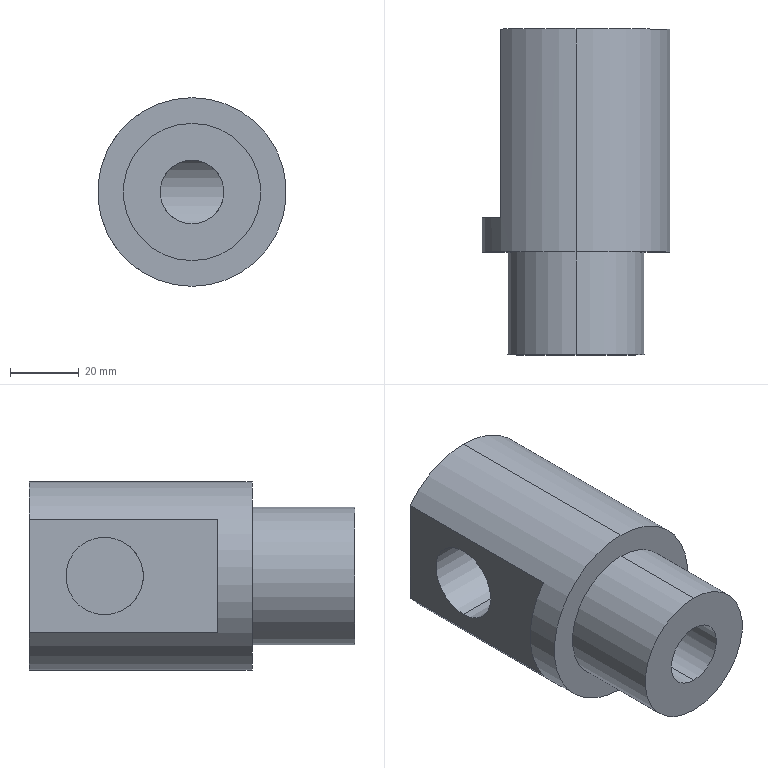Part | SolidWorks | features ICE 4, Extrusion 1 | 1 solid | 14 faces | box 55 x 95 x 55 mm | volume 152228 mm3 | cylinder 8 | plane 6 | commonest cylinder face diameters 18.6 x2 22.6 x2 40 x2 55 x2
STEP:
#1=CARTESIAN_POINT('',(0.,66.581,9.3));
#2=VERTEX_POINT('',#1);
#3=CARTESIAN_POINT('',(0.,66.581,-9.3));
#4=VERTEX_POINT('',#3);
#5=CARTESIAN_POINT('',(0.,66.581,9.3));
#6=CARTESIAN_POINT('',(-0.3235,66.581,9.3));
#7=CARTESIAN_POINT('',(-0.645,66.557,9.283));
#8=CARTESIAN_POINT('',(-1.284,66.462,9.216));
#9=CARTESIAN_POINT('',(-1.603,66.391,9.166));
#10=CARTESIAN_POINT('',(-2.214,66.216,9.038));
#11=CARTESIAN_POINT('',(-2.51,66.113,8.96));
#12=CARTESIAN_POINT('',(-3.087,65.882,8.778));
#13=CARTESIAN_POINT('',(-3.369,65.755,8.673));
#14=CARTESIAN_POINT('',(-4.189,65.35,8.325));
#15=CARTESIAN_POINT('',(-4.693,65.057,8.049));
#16=CARTESIAN_POINT('',(-5.406,64.61,7.573));
#17=CARTESIAN_POINT('',(-5.636,64.46,7.403));
#18=CARTESIAN_POINT('',(-6.081,64.159,7.042));
#19=CARTESIAN_POINT('',(-6.298,64.009,6.849));
#20=CARTESIAN_POINT('',(-6.919,63.567,6.241));
#21=CARTESIAN_POINT('',(-7.294,63.287,5.8));
#22=CARTESIAN_POINT('',(-7.798,62.9,5.076));
#23=CARTESIAN_POINT('',(-7.957,62.777,4.824));
#24=CARTESIAN_POINT('',(-8.253,62.545,4.297));
#25=CARTESIAN_POINT('',(-8.392,62.435,4.021));
#26=CARTESIAN_POINT('',(-8.765,62.137,3.169));
#27=CARTESIAN_POINT('',(-8.96,61.978,2.573));
#28=CARTESIAN_POINT('',(-9.161,61.814,1.632));
#29=CARTESIAN_POINT('',(-9.213,61.772,1.31));
#30=CARTESIAN_POINT('',(-9.282,61.715,0.6676));
#31=CARTESIAN_POINT('',(-9.299,61.701,0.3458));
#32=CARTESIAN_POINT('',(-9.301,61.699,-0.2993));
#33=CARTESIAN_POINT('',(-9.285,61.712,-0.6227));
#34=CARTESIAN_POINT('',(-9.218,61.767,-1.271));
#35=CARTESIAN_POINT('',(-9.168,61.808,-1.592));
#36=CARTESIAN_POINT('',(-9.037,61.915,-2.217));
#37=CARTESIAN_POINT('',(-8.957,61.981,-2.524));
#38=CARTESIAN_POINT('',(-8.765,62.136,-3.125));
#39=CARTESIAN_POINT('',(-8.654,62.226,-3.421));
#40=CARTESIAN_POINT('',(-8.283,62.522,-4.275));
#41=CARTESIAN_POINT('',(-7.987,62.756,-4.802));
#42=CARTESIAN_POINT('',(-7.476,63.147,-5.539));
#43=CARTESIAN_POINT('',(-7.295,63.284,-5.775));
#44=CARTESIAN_POINT('',(-6.918,63.564,-6.222));
#45=CARTESIAN_POINT('',(-6.721,63.707,-6.434));
#46=CARTESIAN_POINT('',(-6.106,64.146,-7.038));
#47=CARTESIAN_POINT('',(-5.664,64.448,-7.399));
#48=CARTESIAN_POINT('',(-4.944,64.9,-7.882));
#49=CARTESIAN_POINT('',(-4.696,65.05,-8.033));
#50=CARTESIAN_POINT('',(-4.186,65.34,-8.31));
#51=CARTESIAN_POINT('',(-3.924,65.48,-8.437));
#52=CARTESIAN_POINT('',(-3.383,65.748,-8.668));
#53=CARTESIAN_POINT('',(-3.104,65.875,-8.772));
#54=CARTESIAN_POINT('',(-2.524,66.108,-8.956));
#55=CARTESIAN_POINT('',(-2.223,66.214,-9.036));
#56=CARTESIAN_POINT('',(-1.611,66.389,-9.165));
#57=CARTESIAN_POINT('',(-1.298,66.459,-9.215));
#58=CARTESIAN_POINT('',(-0.6581,66.555,-9.282));
#59=CARTESIAN_POINT('',(-0.3284,66.581,-9.3));
#60=CARTESIAN_POINT('',(0.,66.581,-9.3));
#61=B_SPLINE_CURVE_WITH_KNOTS('',3,(#5,#6,#7,#8,#9,#10,#11,#12,#13,#14,#15,#16,#17,#18,#19,#20,#21,#22,#23,#24,#25,#26,#27,#28,#29,#30,#31,#32,#33,#34,#35,#36,#37,#38,#39,#40,#41,#42,#43,#44,#45,#46,#47,#48,#49,#50,#51,#52,#53,#54,#55,#56,#57,#58,#59,#60),.UNSPECIFIED.,.F.,.F.,(4,2,2,2,2,2,2,2,2,2,2,2,2,2,2,2,2,2,2,2,2,2,2,2,2,2,2,4),(0.03102,0.03199,0.03295,0.03392,0.03489,0.03683,0.0378,0.03877,0.04071,0.04167,0.04264,0.04458,0.04555,0.04652,0.04749,0.04846,0.04943,0.05039,0.05233,0.0533,0.05427,0.05621,0.05718,0.05814,0.05911,0.06008,0.06105,0.06202),.UNSPECIFIED.);
#62=EDGE_CURVE('',#2,#4,#61,.T.);
#63=ORIENTED_EDGE('',*,*,#62,.F.);
#64=CARTESIAN_POINT('',(0.,0.,9.3));
#65=VERTEX_POINT('',#64);
#66=CARTESIAN_POINT('',(0.,74.,9.3));
#67=DIRECTION('',(0.,-1.,0.));
#68=VECTOR('',#67,1000.);
#69=LINE('',#66,#68);
#70=EDGE_CURVE('',#2,#65,#69,.T.);
#71=ORIENTED_EDGE('',*,*,#70,.T.);
#72=CARTESIAN_POINT('',(0.,0.,-9.3));
#73=VERTEX_POINT('',#72);
#74=CARTESIAN_POINT('',(0.,0.,0.));
#75=DIRECTION('',(0.,-1.,0.));
#76=DIRECTION('',(0.,0.,-1.));
#77=AXIS2_PLACEMENT_3D('',#74,#75,#76);
#78=CIRCLE('',#77,9.3);
#79=EDGE_CURVE('',#65,#73,#78,.T.);
#80=ORIENTED_EDGE('',*,*,#79,.T.);
#81=CARTESIAN_POINT('',(0.,74.,-9.3));
#82=DIRECTION('',(0.,-1.,0.));
#83=VECTOR('',#82,1000.);
#84=LINE('',#81,#83);
#85=EDGE_CURVE('',#4,#73,#84,.T.);
#86=ORIENTED_EDGE('',*,*,#85,.F.);
#87=EDGE_LOOP('',(#63,#71,#80,#86));
#88=FACE_OUTER_BOUND('',#87,.T.);
#89=CARTESIAN_POINT('',(0.,74.,0.));
#90=DIRECTION('',(0.,-1.,0.));
#91=DIRECTION('',(0.,0.,-1.));
#92=AXIS2_PLACEMENT_3D('',#89,#90,#91);
#93=CYLINDRICAL_SURFACE('',#92,9.3);
#94=ADVANCED_FACE('',(#88),#93,.F.);
#95=CARTESIAN_POINT('',(0.,66.581,-9.3));
#96=CARTESIAN_POINT('',(0.6571,66.581,-9.3));
#97=CARTESIAN_POINT('',(1.292,66.479,-9.231));
#98=CARTESIAN_POINT('',(2.525,66.128,-8.973));
#99=CARTESIAN_POINT('',(3.099,65.888,-8.788));
#100=CARTESIAN_POINT('',(4.183,65.353,-8.327));
#101=CARTESIAN_POINT('',(4.697,65.055,-8.047));
#102=CARTESIAN_POINT('',(5.648,64.458,-7.411));
#103=CARTESIAN_POINT('',(6.089,64.157,-7.053));
#104=CARTESIAN_POINT('',(6.912,63.571,-6.248));
#105=CARTESIAN_POINT('',(7.296,63.285,-5.797));
#106=CARTESIAN_POINT('',(7.972,62.767,-4.825));
#107=CARTESIAN_POINT('',(8.269,62.534,-4.302));
#108=CARTESIAN_POINT('',(8.642,62.235,-3.449));
#109=CARTESIAN_POINT('',(8.754,62.145,-3.155));
#110=CARTESIAN_POINT('',(8.947,61.989,-2.557));
#111=CARTESIAN_POINT('',(9.029,61.922,-2.252));
#112=CARTESIAN_POINT('',(9.162,61.814,-1.629));
#113=CARTESIAN_POINT('',(9.213,61.771,-1.309));
#114=CARTESIAN_POINT('',(9.282,61.715,-0.6616));
#115=CARTESIAN_POINT('',(9.299,61.7,-0.3386));
#116=CARTESIAN_POINT('',(9.301,61.7,0.3063));
#117=CARTESIAN_POINT('',(9.284,61.713,0.6282));
#118=CARTESIAN_POINT('',(9.218,61.767,1.271));
#119=CARTESIAN_POINT('',(9.168,61.808,1.594));
#120=CARTESIAN_POINT('',(8.971,61.97,2.535));
#121=CARTESIAN_POINT('',(8.779,62.126,3.133));
#122=CARTESIAN_POINT('',(8.282,62.523,4.276));
#123=CARTESIAN_POINT('',(7.986,62.757,4.803));
#124=CARTESIAN_POINT('',(7.478,63.146,5.537));
#125=CARTESIAN_POINT('',(7.297,63.282,5.773));
#126=CARTESIAN_POINT('',(6.918,63.564,6.222));
#127=CARTESIAN_POINT('',(6.72,63.708,6.435));
#128=CARTESIAN_POINT('',(6.103,64.148,7.041));
#129=CARTESIAN_POINT('',(5.659,64.451,7.403));
#130=CARTESIAN_POINT('',(4.698,65.054,8.047));
#131=CARTESIAN_POINT('',(4.19,65.349,8.323));
#132=CARTESIAN_POINT('',(3.379,65.75,8.67));
#133=CARTESIAN_POINT('',(3.099,65.877,8.774));
#134=CARTESIAN_POINT('',(2.519,66.11,8.958));
#135=CARTESIAN_POINT('',(2.218,66.215,9.037));
#136=CARTESIAN_POINT('',(1.606,66.39,9.166));
#137=CARTESIAN_POINT('',(1.294,66.46,9.215));
#138=CARTESIAN_POINT('',(0.6525,66.556,9.283));
#139=CARTESIAN_POINT('',(0.3236,66.581,9.3));
#140=CARTESIAN_POINT('',(0.,66.581,9.3));
#141=B_SPLINE_CURVE_WITH_KNOTS('',3,(#95,#96,#97,#98,#99,#100,#101,#102,#103,#104,#105,#106,#107,#108,#109,#110,#111,#112,#113,#114,#115,#116,#117,#118,#119,#120,#121,#122,#123,#124,#125,#126,#127,#128,#129,#130,#131,#132,#133,#134,#135,#136,#137,#138,#139,#140),.UNSPECIFIED.,.F.,.F.,(4,2,2,2,2,2,2,2,2,2,2,2,2,2,2,2,2,2,2,2,2,2,4),(0.,0.001939,0.003877,0.005816,0.007754,0.009693,0.01163,0.0126,0.01357,0.01454,0.01551,0.01648,0.01745,0.01939,0.02132,0.02229,0.02326,0.0252,0.02714,0.02811,0.02908,0.03005,0.03102),.UNSPECIFIED.);
#142=EDGE_CURVE('',#4,#2,#141,.T.);
#143=ORIENTED_EDGE('',*,*,#142,.T.);
#144=ORIENTED_EDGE('',*,*,#62,.T.);
#145=EDGE_LOOP('',(#143,#144));
#146=FACE_BOUND('',#145,.T.);
#147=CARTESIAN_POINT('',(18.,73.,-11.3));
#148=VERTEX_POINT('',#147);
#149=CARTESIAN_POINT('',(18.,73.,11.3));
#150=VERTEX_POINT('',#149);
#151=CARTESIAN_POINT('',(18.,73.,0.));
#152=DIRECTION('',(-1.,0.,0.));
#153=DIRECTION('',(0.,0.,1.));
#154=AXIS2_PLACEMENT_3D('',#151,#152,#153);
#155=CIRCLE('',#154,11.3);
#156=EDGE_CURVE('',#148,#150,#155,.T.);
#157=ORIENTED_EDGE('',*,*,#156,.F.);
#158=CARTESIAN_POINT('',(-22.,73.,-11.3));
#159=VERTEX_POINT('',#158);
#160=CARTESIAN_POINT('',(18.,73.,-11.3));
#161=DIRECTION('',(-1.,0.,0.));
#162=VECTOR('',#161,1000.);
#163=LINE('',#160,#162);
#164=EDGE_CURVE('',#148,#159,#163,.T.);
#165=ORIENTED_EDGE('',*,*,#164,.T.);
#166=CARTESIAN_POINT('',(-22.,73.,11.3));
#167=VERTEX_POINT('',#166);
#168=CARTESIAN_POINT('',(-22.,73.,0.));
#169=DIRECTION('',(-1.,0.,0.));
#170=DIRECTION('',(0.,0.,1.));
#171=AXIS2_PLACEMENT_3D('',#168,#169,#170);
#172=CIRCLE('',#171,11.3);
#173=EDGE_CURVE('',#159,#167,#172,.T.);
#174=ORIENTED_EDGE('',*,*,#173,.T.);
#175=CARTESIAN_POINT('',(18.,73.,11.3));
#176=DIRECTION('',(-1.,0.,0.));
#177=VECTOR('',#176,1000.);
#178=LINE('',#175,#177);
#179=EDGE_CURVE('',#150,#167,#178,.T.);
#180=ORIENTED_EDGE('',*,*,#179,.F.);
#181=EDGE_LOOP('',(#157,#165,#174,#180));
#182=FACE_OUTER_BOUND('',#181,.T.);
#183=CARTESIAN_POINT('',(18.,73.,0.));
#184=DIRECTION('',(-1.,0.,0.));
#185=DIRECTION('',(0.,0.,1.));
#186=AXIS2_PLACEMENT_3D('',#183,#184,#185);
#187=CYLINDRICAL_SURFACE('',#186,11.3);
#188=ADVANCED_FACE('',(#146,#182),#187,.F.);
#189=CARTESIAN_POINT('',(0.,95.,27.5));
#190=VERTEX_POINT('',#189);
#191=CARTESIAN_POINT('',(0.,95.,-27.5));
#192=VERTEX_POINT('',#191);
#193=CARTESIAN_POINT('',(0.,95.,0.));
#194=DIRECTION('',(0.,1.,0.));
#195=DIRECTION('',(0.,0.,1.));
#196=AXIS2_PLACEMENT_3D('',#193,#194,#195);
#197=CIRCLE('',#196,27.5);
#198=EDGE_CURVE('',#190,#192,#197,.T.);
#199=ORIENTED_EDGE('',*,*,#198,.F.);
#200=CARTESIAN_POINT('',(0.,30.,27.5));
#201=VERTEX_POINT('',#200);
#202=CARTESIAN_POINT('',(0.,95.,27.5));
#203=DIRECTION('',(0.,-1.,0.));
#204=VECTOR('',#203,1000.);
#205=LINE('',#202,#204);
#206=EDGE_CURVE('',#190,#201,#205,.T.);
#207=ORIENTED_EDGE('',*,*,#206,.T.);
#208=CARTESIAN_POINT('',(0.,30.,-27.5));
#209=VERTEX_POINT('',#208);
#210=CARTESIAN_POINT('',(0.,30.,0.));
#211=DIRECTION('',(0.,1.,0.));
#212=DIRECTION('',(0.,0.,1.));
#213=AXIS2_PLACEMENT_3D('',#210,#211,#212);
#214=CIRCLE('',#213,27.5);
#215=EDGE_CURVE('',#201,#209,#214,.T.);
#216=ORIENTED_EDGE('',*,*,#215,.T.);
#217=CARTESIAN_POINT('',(0.,95.,-27.5));
#218=DIRECTION('',(0.,-1.,0.));
#219=VECTOR('',#218,1000.);
#220=LINE('',#217,#219);
#221=EDGE_CURVE('',#192,#209,#220,.T.);
#222=ORIENTED_EDGE('',*,*,#221,.F.);
#223=EDGE_LOOP('',(#199,#207,#216,#222));
#224=FACE_OUTER_BOUND('',#223,.T.);
#225=CARTESIAN_POINT('',(0.,95.,0.));
#226=DIRECTION('',(0.,-1.,0.));
#227=DIRECTION('',(0.,0.,-1.));
#228=AXIS2_PLACEMENT_3D('',#225,#226,#227);
#229=CYLINDRICAL_SURFACE('',#228,27.5);
#230=ADVANCED_FACE('',(#224),#229,.T.);
#231=CARTESIAN_POINT('',(0.,30.,20.));
#232=VERTEX_POINT('',#231);
#233=CARTESIAN_POINT('',(0.,30.,-20.));
#234=VERTEX_POINT('',#233);
#235=CARTESIAN_POINT('',(0.,30.,0.));
#236=DIRECTION('',(0.,1.,0.));
#237=DIRECTION('',(0.,0.,1.));
#238=AXIS2_PLACEMENT_3D('',#235,#236,#237);
#239=CIRCLE('',#238,20.);
#240=EDGE_CURVE('',#232,#234,#239,.T.);
#241=ORIENTED_EDGE('',*,*,#240,.F.);
#242=CARTESIAN_POINT('',(0.,0.,20.));
#243=VERTEX_POINT('',#242);
#244=CARTESIAN_POINT('',(0.,30.,20.));
#245=DIRECTION('',(0.,-1.,0.));
#246=VECTOR('',#245,1000.);
#247=LINE('',#244,#246);
#248=EDGE_CURVE('',#232,#243,#247,.T.);
#249=ORIENTED_EDGE('',*,*,#248,.T.);
#250=CARTESIAN_POINT('',(0.,0.,-20.));
#251=VERTEX_POINT('',#250);
#252=CARTESIAN_POINT('',(0.,0.,0.));
#253=DIRECTION('',(0.,1.,0.));
#254=DIRECTION('',(0.,0.,1.));
#255=AXIS2_PLACEMENT_3D('',#252,#253,#254);
#256=CIRCLE('',#255,20.);
#257=EDGE_CURVE('',#243,#251,#256,.T.);
#258=ORIENTED_EDGE('',*,*,#257,.T.);
#259=CARTESIAN_POINT('',(0.,30.,-20.));
#260=DIRECTION('',(0.,-1.,0.));
#261=VECTOR('',#260,1000.);
#262=LINE('',#259,#261);
#263=EDGE_CURVE('',#234,#251,#262,.T.);
#264=ORIENTED_EDGE('',*,*,#263,.F.);
#265=EDGE_LOOP('',(#241,#249,#258,#264));
#266=FACE_OUTER_BOUND('',#265,.T.);
#267=CARTESIAN_POINT('',(0.,30.,0.));
#268=DIRECTION('',(0.,-1.,0.));
#269=DIRECTION('',(0.,0.,-1.));
#270=AXIS2_PLACEMENT_3D('',#267,#268,#269);
#271=CYLINDRICAL_SURFACE('',#270,20.);
#272=ADVANCED_FACE('',(#266),#271,.T.);
#273=ORIENTED_EDGE('',*,*,#248,.F.);
#274=CARTESIAN_POINT('',(0.,30.,0.));
#275=DIRECTION('',(0.,1.,0.));
#276=DIRECTION('',(0.,0.,1.));
#277=AXIS2_PLACEMENT_3D('',#274,#275,#276);
#278=CIRCLE('',#277,20.);
#279=EDGE_CURVE('',#234,#232,#278,.T.);
#280=ORIENTED_EDGE('',*,*,#279,.F.);
#281=ORIENTED_EDGE('',*,*,#263,.T.);
#282=CARTESIAN_POINT('',(0.,0.,0.));
#283=DIRECTION('',(0.,1.,0.));
#284=DIRECTION('',(0.,0.,1.));
#285=AXIS2_PLACEMENT_3D('',#282,#283,#284);
#286=CIRCLE('',#285,20.);
#287=EDGE_CURVE('',#251,#243,#286,.T.);
#288=ORIENTED_EDGE('',*,*,#287,.T.);
#289=EDGE_LOOP('',(#273,#280,#281,#288));
#290=FACE_OUTER_BOUND('',#289,.T.);
#291=CARTESIAN_POINT('',(0.,30.,0.));
#292=DIRECTION('',(0.,-1.,0.));
#293=DIRECTION('',(0.,0.,-1.));
#294=AXIS2_PLACEMENT_3D('',#291,#292,#293);
#295=CYLINDRICAL_SURFACE('',#294,20.);
#296=ADVANCED_FACE('',(#290),#295,.T.);
#297=CARTESIAN_POINT('',(0.,0.,0.));
#298=DIRECTION('',(0.,-1.,0.));
#299=DIRECTION('',(0.,0.,-1.));
#300=AXIS2_PLACEMENT_3D('',#297,#298,#299);
#301=CIRCLE('',#300,9.3);
#302=EDGE_CURVE('',#73,#65,#301,.T.);
#303=ORIENTED_EDGE('',*,*,#302,.F.);
#304=ORIENTED_EDGE('',*,*,#79,.F.);
#305=EDGE_LOOP('',(#303,#304));
#306=FACE_BOUND('',#305,.T.);
#307=ORIENTED_EDGE('',*,*,#287,.F.);
#308=ORIENTED_EDGE('',*,*,#257,.F.);
#309=EDGE_LOOP('',(#307,#308));
#310=FACE_OUTER_BOUND('',#309,.T.);
#311=CARTESIAN_POINT('',(0.,0.,0.));
#312=DIRECTION('',(0.,1.,0.));
#313=DIRECTION('',(0.,0.,1.));
#314=AXIS2_PLACEMENT_3D('',#311,#312,#313);
#315=PLANE('',#314);
#316=ADVANCED_FACE('',(#306,#310),#315,.F.);
#317=ORIENTED_EDGE('',*,*,#206,.F.);
#318=CARTESIAN_POINT('',(-22.,95.,16.5));
#319=VERTEX_POINT('',#318);
#320=CARTESIAN_POINT('',(0.,95.,0.));
#321=DIRECTION('',(0.,1.,0.));
#322=DIRECTION('',(0.,0.,1.));
#323=AXIS2_PLACEMENT_3D('',#320,#321,#322);
#324=CIRCLE('',#323,27.5);
#325=EDGE_CURVE('',#319,#190,#324,.T.);
#326=ORIENTED_EDGE('',*,*,#325,.F.);
#327=CARTESIAN_POINT('',(-22.,40.,16.5));
#328=VERTEX_POINT('',#327);
#329=CARTESIAN_POINT('',(-22.,95.,16.5));
#330=DIRECTION('',(0.,-1.,0.));
#331=VECTOR('',#330,1000.);
#332=LINE('',#329,#331);
#333=EDGE_CURVE('',#319,#328,#332,.T.);
#334=ORIENTED_EDGE('',*,*,#333,.T.);
#335=CARTESIAN_POINT('',(-22.,40.,-16.5));
#336=VERTEX_POINT('',#335);
#337=CARTESIAN_POINT('',(0.,40.,0.));
#338=DIRECTION('',(0.,-1.,0.));
#339=DIRECTION('',(0.,0.,-1.));
#340=AXIS2_PLACEMENT_3D('',#337,#338,#339);
#341=CIRCLE('',#340,27.5);
#342=EDGE_CURVE('',#328,#336,#341,.T.);
#343=ORIENTED_EDGE('',*,*,#342,.T.);
#344=CARTESIAN_POINT('',(-22.,95.,-16.5));
#345=VERTEX_POINT('',#344);
#346=CARTESIAN_POINT('',(-22.,95.,-16.5));
#347=DIRECTION('',(0.,1.,0.));
#348=VECTOR('',#347,1000.);
#349=LINE('',#346,#348);
#350=EDGE_CURVE('',#336,#345,#349,.T.);
#351=ORIENTED_EDGE('',*,*,#350,.T.);
#352=CARTESIAN_POINT('',(0.,95.,0.));
#353=DIRECTION('',(0.,1.,0.));
#354=DIRECTION('',(0.,0.,1.));
#355=AXIS2_PLACEMENT_3D('',#352,#353,#354);
#356=CIRCLE('',#355,27.5);
#357=EDGE_CURVE('',#192,#345,#356,.T.);
#358=ORIENTED_EDGE('',*,*,#357,.F.);
#359=ORIENTED_EDGE('',*,*,#221,.T.);
#360=CARTESIAN_POINT('',(0.,30.,0.));
#361=DIRECTION('',(0.,1.,0.));
#362=DIRECTION('',(0.,0.,1.));
#363=AXIS2_PLACEMENT_3D('',#360,#361,#362);
#364=CIRCLE('',#363,27.5);
#365=EDGE_CURVE('',#209,#201,#364,.T.);
#366=ORIENTED_EDGE('',*,*,#365,.T.);
#367=EDGE_LOOP('',(#317,#326,#334,#343,#351,#358,#359,#366));
#368=FACE_OUTER_BOUND('',#367,.T.);
#369=CARTESIAN_POINT('',(0.,95.,0.));
#370=DIRECTION('',(0.,-1.,0.));
#371=DIRECTION('',(0.,0.,-1.));
#372=AXIS2_PLACEMENT_3D('',#369,#370,#371);
#373=CYLINDRICAL_SURFACE('',#372,27.5);
#374=ADVANCED_FACE('',(#368),#373,.T.);
#375=CARTESIAN_POINT('',(-22.,95.,0.));
#376=DIRECTION('',(0.,0.,-1.));
#377=VECTOR('',#376,1000.);
#378=LINE('',#375,#377);
#379=EDGE_CURVE('',#319,#345,#378,.T.);
#380=ORIENTED_EDGE('',*,*,#379,.F.);
#381=ORIENTED_EDGE('',*,*,#325,.T.);
#382=ORIENTED_EDGE('',*,*,#198,.T.);
#383=ORIENTED_EDGE('',*,*,#357,.T.);
#384=EDGE_LOOP('',(#380,#381,#382,#383));
#385=FACE_OUTER_BOUND('',#384,.T.);
#386=CARTESIAN_POINT('',(0.,95.,0.));
#387=DIRECTION('',(0.,1.,0.));
#388=DIRECTION('',(0.,0.,1.));
#389=AXIS2_PLACEMENT_3D('',#386,#387,#388);
#390=PLANE('',#389);
#391=ADVANCED_FACE('',(#385),#390,.T.);
#392=ORIENTED_EDGE('',*,*,#279,.T.);
#393=ORIENTED_EDGE('',*,*,#240,.T.);
#394=EDGE_LOOP('',(#392,#393));
#395=FACE_BOUND('',#394,.T.);
#396=ORIENTED_EDGE('',*,*,#365,.F.);
#397=ORIENTED_EDGE('',*,*,#215,.F.);
#398=EDGE_LOOP('',(#396,#397));
#399=FACE_OUTER_BOUND('',#398,.T.);
#400=CARTESIAN_POINT('',(0.,30.,0.));
#401=DIRECTION('',(0.,1.,0.));
#402=DIRECTION('',(0.,0.,1.));
#403=AXIS2_PLACEMENT_3D('',#400,#401,#402);
#404=PLANE('',#403);
#405=ADVANCED_FACE('',(#395,#399),#404,.F.);
#406=CARTESIAN_POINT('',(-22.,40.,17.5));
#407=DIRECTION('',(0.,0.,-1.));
#408=VECTOR('',#407,1000.);
#409=LINE('',#406,#408);
#410=EDGE_CURVE('',#328,#336,#409,.T.);
#411=ORIENTED_EDGE('',*,*,#410,.T.);
#412=ORIENTED_EDGE('',*,*,#342,.F.);
#413=EDGE_LOOP('',(#411,#412));
#414=FACE_OUTER_BOUND('',#413,.T.);
#415=CARTESIAN_POINT('',(-87.,40.,17.5));
#416=DIRECTION('',(0.,-1.,0.));
#417=DIRECTION('',(0.,0.,-1.));
#418=AXIS2_PLACEMENT_3D('',#415,#416,#417);
#419=PLANE('',#418);
#420=ADVANCED_FACE('',(#414),#419,.F.);
#421=CARTESIAN_POINT('',(-22.,73.,0.));
#422=DIRECTION('',(-1.,0.,0.));
#423=DIRECTION('',(0.,0.,1.));
#424=AXIS2_PLACEMENT_3D('',#421,#422,#423);
#425=CIRCLE('',#424,11.3);
#426=EDGE_CURVE('',#167,#159,#425,.T.);
#427=ORIENTED_EDGE('',*,*,#426,.F.);
#428=ORIENTED_EDGE('',*,*,#173,.F.);
#429=EDGE_LOOP('',(#427,#428));
#430=FACE_BOUND('',#429,.T.);
#431=ORIENTED_EDGE('',*,*,#379,.T.);
#432=ORIENTED_EDGE('',*,*,#350,.F.);
#433=ORIENTED_EDGE('',*,*,#410,.F.);
#434=ORIENTED_EDGE('',*,*,#333,.F.);
#435=EDGE_LOOP('',(#431,#432,#433,#434));
#436=FACE_OUTER_BOUND('',#435,.T.);
#437=CARTESIAN_POINT('',(-22.,0.,0.));
#438=DIRECTION('',(1.,0.,0.));
#439=DIRECTION('',(0.,0.,-1.));
#440=AXIS2_PLACEMENT_3D('',#437,#438,#439);
#441=PLANE('',#440);
#442=ADVANCED_FACE('',(#430,#436),#441,.F.);
#443=ORIENTED_EDGE('',*,*,#164,.F.);
#444=CARTESIAN_POINT('',(18.,73.,0.));
#445=DIRECTION('',(-1.,0.,0.));
#446=DIRECTION('',(0.,0.,1.));
#447=AXIS2_PLACEMENT_3D('',#444,#445,#446);
#448=CIRCLE('',#447,11.3);
#449=EDGE_CURVE('',#150,#148,#448,.T.);
#450=ORIENTED_EDGE('',*,*,#449,.F.);
#451=ORIENTED_EDGE('',*,*,#179,.T.);
#452=ORIENTED_EDGE('',*,*,#426,.T.);
#453=EDGE_LOOP('',(#443,#450,#451,#452));
#454=FACE_OUTER_BOUND('',#453,.T.);
#455=CARTESIAN_POINT('',(18.,73.,0.));
#456=DIRECTION('',(-1.,0.,0.));
#457=DIRECTION('',(0.,0.,1.));
#458=AXIS2_PLACEMENT_3D('',#455,#456,#457);
#459=CYLINDRICAL_SURFACE('',#458,11.3);
#460=ADVANCED_FACE('',(#454),#459,.F.);
#461=ORIENTED_EDGE('',*,*,#449,.T.);
#462=ORIENTED_EDGE('',*,*,#156,.T.);
#463=EDGE_LOOP('',(#461,#462));
#464=FACE_OUTER_BOUND('',#463,.T.);
#465=CARTESIAN_POINT('',(18.,73.,0.));
#466=DIRECTION('',(-1.,0.,0.));
#467=DIRECTION('',(0.,0.,1.));
#468=AXIS2_PLACEMENT_3D('',#465,#466,#467);
#469=PLANE('',#468);
#470=ADVANCED_FACE('',(#464),#469,.T.);
#471=ORIENTED_EDGE('',*,*,#70,.F.);
#472=ORIENTED_EDGE('',*,*,#142,.F.);
#473=ORIENTED_EDGE('',*,*,#85,.T.);
#474=ORIENTED_EDGE('',*,*,#302,.T.);
#475=EDGE_LOOP('',(#471,#472,#473,#474));
#476=FACE_OUTER_BOUND('',#475,.T.);
#477=CARTESIAN_POINT('',(0.,74.,0.));
#478=DIRECTION('',(0.,-1.,0.));
#479=DIRECTION('',(0.,0.,-1.));
#480=AXIS2_PLACEMENT_3D('',#477,#478,#479);
#481=CYLINDRICAL_SURFACE('',#480,9.3);
#482=ADVANCED_FACE('',(#476),#481,.F.);
#483=CLOSED_SHELL('',(#94,#188,#230,#272,#296,#316,#374,#391,#405,#420,#442,#460,#470,#482));
#484=MANIFOLD_SOLID_BREP('',#483);
#485=CARTESIAN_POINT('',(0.,0.,0.));
#486=DIRECTION('',(0.,0.,1.));
#487=DIRECTION('',(1.,0.,0.));
#488=AXIS2_PLACEMENT_3D('',#485,#486,#487);
#489=(LENGTH_UNIT()NAMED_UNIT(*)SI_UNIT(.MILLI.,.METRE.));
#490=UNCERTAINTY_MEASURE_WITH_UNIT(LENGTH_MEASURE(0.00001),#489,'','');
#491=(NAMED_UNIT(*)PLANE_ANGLE_UNIT()SI_UNIT($,.RADIAN.));
#492=(NAMED_UNIT(*)SI_UNIT($,.STERADIAN.)SOLID_ANGLE_UNIT());
#493=(GEOMETRIC_REPRESENTATION_CONTEXT(3)GLOBAL_UNCERTAINTY_ASSIGNED_CONTEXT((#490))GLOBAL_UNIT_ASSIGNED_CONTEXT((#489,#491,#492))REPRESENTATION_CONTEXT('',''));
#494=ADVANCED_BREP_SHAPE_REPRESENTATION('',(#484,#488),#493);